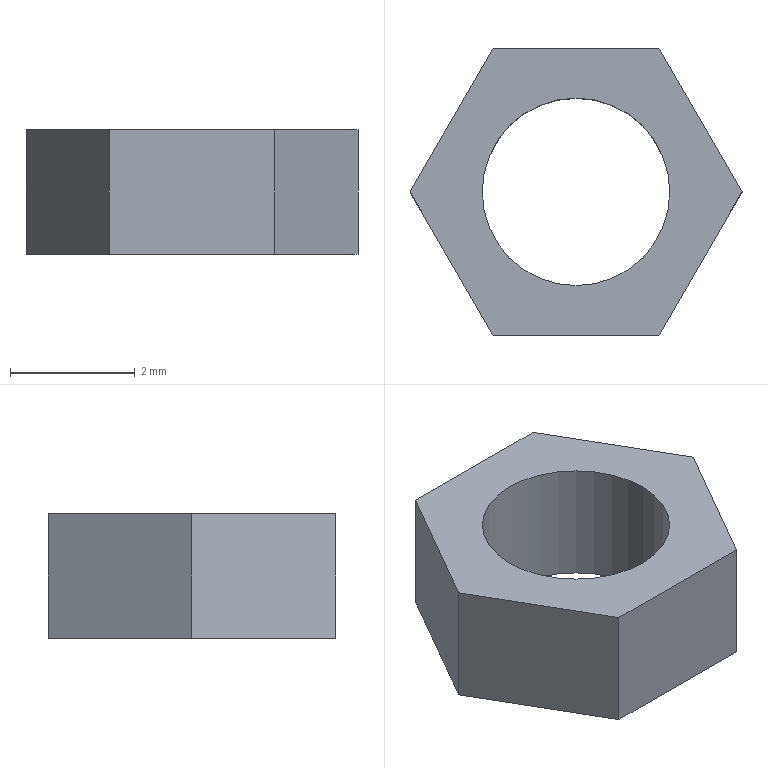Part | SolidWorks | features BaseBody 1 | 1 solid | 10 faces | box 5.314 x 4.602 x 2 mm | volume 22.552 mm3 | plane 8 | cylinder 2 | commonest cylinder face diameters 3 x2
STEP:
#1=CARTESIAN_POINT('',(35.309,0.,0.));
#2=VERTEX_POINT('',#1);
#3=CARTESIAN_POINT('',(38.309,0.,0.));
#4=VERTEX_POINT('',#3);
#5=CARTESIAN_POINT('',(36.809,0.,0.));
#6=DIRECTION('',(0.,0.,1.));
#7=DIRECTION('',(1.,0.,0.));
#8=AXIS2_PLACEMENT_3D('',#5,#6,#7);
#9=CIRCLE('',#8,1.5);
#10=EDGE_CURVE('',#2,#4,#9,.T.);
#11=ORIENTED_EDGE('',*,*,#10,.F.);
#12=CARTESIAN_POINT('',(35.309,0.,2.));
#13=VERTEX_POINT('',#12);
#14=CARTESIAN_POINT('',(35.309,0.,0.));
#15=DIRECTION('',(0.,0.,1.));
#16=VECTOR('',#15,1000.);
#17=LINE('',#14,#16);
#18=EDGE_CURVE('',#2,#13,#17,.T.);
#19=ORIENTED_EDGE('',*,*,#18,.T.);
#20=CARTESIAN_POINT('',(38.309,0.,2.));
#21=VERTEX_POINT('',#20);
#22=CARTESIAN_POINT('',(36.809,0.,2.));
#23=DIRECTION('',(0.,0.,-1.));
#24=DIRECTION('',(1.,0.,0.));
#25=AXIS2_PLACEMENT_3D('',#22,#23,#24);
#26=CIRCLE('',#25,1.5);
#27=EDGE_CURVE('',#21,#13,#26,.T.);
#28=ORIENTED_EDGE('',*,*,#27,.F.);
#29=CARTESIAN_POINT('',(38.309,0.,0.));
#30=DIRECTION('',(0.,0.,1.));
#31=VECTOR('',#30,1000.);
#32=LINE('',#29,#31);
#33=EDGE_CURVE('',#4,#21,#32,.T.);
#34=ORIENTED_EDGE('',*,*,#33,.F.);
#35=EDGE_LOOP('',(#11,#19,#28,#34));
#36=FACE_OUTER_BOUND('',#35,.T.);
#37=CARTESIAN_POINT('',(36.809,0.,0.));
#38=DIRECTION('',(0.,0.,1.));
#39=DIRECTION('',(1.,0.,0.));
#40=AXIS2_PLACEMENT_3D('',#37,#38,#39);
#41=CYLINDRICAL_SURFACE('',#40,1.5);
#42=ADVANCED_FACE('',(#36),#41,.F.);
#43=ORIENTED_EDGE('',*,*,#18,.F.);
#44=CARTESIAN_POINT('',(36.809,0.,0.));
#45=DIRECTION('',(0.,0.,1.));
#46=DIRECTION('',(1.,0.,0.));
#47=AXIS2_PLACEMENT_3D('',#44,#45,#46);
#48=CIRCLE('',#47,1.5);
#49=EDGE_CURVE('',#4,#2,#48,.T.);
#50=ORIENTED_EDGE('',*,*,#49,.F.);
#51=ORIENTED_EDGE('',*,*,#33,.T.);
#52=CARTESIAN_POINT('',(36.809,0.,2.));
#53=DIRECTION('',(0.,0.,-1.));
#54=DIRECTION('',(1.,0.,0.));
#55=AXIS2_PLACEMENT_3D('',#52,#53,#54);
#56=CIRCLE('',#55,1.5);
#57=EDGE_CURVE('',#13,#21,#56,.T.);
#58=ORIENTED_EDGE('',*,*,#57,.F.);
#59=EDGE_LOOP('',(#43,#50,#51,#58));
#60=FACE_OUTER_BOUND('',#59,.T.);
#61=CARTESIAN_POINT('',(36.809,0.,0.));
#62=DIRECTION('',(0.,0.,1.));
#63=DIRECTION('',(1.,0.,0.));
#64=AXIS2_PLACEMENT_3D('',#61,#62,#63);
#65=CYLINDRICAL_SURFACE('',#64,1.5);
#66=ADVANCED_FACE('',(#60),#65,.F.);
#67=ORIENTED_EDGE('',*,*,#27,.T.);
#68=ORIENTED_EDGE('',*,*,#57,.T.);
#69=EDGE_LOOP('',(#67,#68));
#70=FACE_BOUND('',#69,.T.);
#71=CARTESIAN_POINT('',(39.466,0.,2.));
#72=VERTEX_POINT('',#71);
#73=CARTESIAN_POINT('',(38.138,2.301,2.));
#74=VERTEX_POINT('',#73);
#75=CARTESIAN_POINT('',(39.466,0.,2.));
#76=DIRECTION('',(-0.5,0.866,0.));
#77=VECTOR('',#76,1000.);
#78=LINE('',#75,#77);
#79=EDGE_CURVE('',#72,#74,#78,.T.);
#80=ORIENTED_EDGE('',*,*,#79,.T.);
#81=CARTESIAN_POINT('',(35.48,2.301,2.));
#82=VERTEX_POINT('',#81);
#83=CARTESIAN_POINT('',(36.809,2.301,2.));
#84=DIRECTION('',(-1.,0.,0.));
#85=VECTOR('',#84,1000.);
#86=LINE('',#83,#85);
#87=EDGE_CURVE('',#74,#82,#86,.T.);
#88=ORIENTED_EDGE('',*,*,#87,.T.);
#89=CARTESIAN_POINT('',(34.152,0.,2.));
#90=VERTEX_POINT('',#89);
#91=CARTESIAN_POINT('',(35.48,2.301,2.));
#92=DIRECTION('',(-0.5,-0.866,0.));
#93=VECTOR('',#92,1000.);
#94=LINE('',#91,#93);
#95=EDGE_CURVE('',#82,#90,#94,.T.);
#96=ORIENTED_EDGE('',*,*,#95,.T.);
#97=CARTESIAN_POINT('',(35.48,-2.301,2.));
#98=VERTEX_POINT('',#97);
#99=CARTESIAN_POINT('',(34.152,0.,2.));
#100=DIRECTION('',(0.5,-0.866,0.));
#101=VECTOR('',#100,1000.);
#102=LINE('',#99,#101);
#103=EDGE_CURVE('',#90,#98,#102,.T.);
#104=ORIENTED_EDGE('',*,*,#103,.T.);
#105=CARTESIAN_POINT('',(38.138,-2.301,2.));
#106=VERTEX_POINT('',#105);
#107=CARTESIAN_POINT('',(36.809,-2.301,2.));
#108=DIRECTION('',(1.,0.,0.));
#109=VECTOR('',#108,1000.);
#110=LINE('',#107,#109);
#111=EDGE_CURVE('',#98,#106,#110,.T.);
#112=ORIENTED_EDGE('',*,*,#111,.T.);
#113=CARTESIAN_POINT('',(38.138,-2.301,2.));
#114=DIRECTION('',(0.5,0.866,0.));
#115=VECTOR('',#114,1000.);
#116=LINE('',#113,#115);
#117=EDGE_CURVE('',#106,#72,#116,.T.);
#118=ORIENTED_EDGE('',*,*,#117,.T.);
#119=EDGE_LOOP('',(#80,#88,#96,#104,#112,#118));
#120=FACE_OUTER_BOUND('',#119,.T.);
#121=CARTESIAN_POINT('',(36.809,0.,2.));
#122=DIRECTION('',(0.,0.,1.));
#123=DIRECTION('',(1.,0.,0.));
#124=AXIS2_PLACEMENT_3D('',#121,#122,#123);
#125=PLANE('',#124);
#126=ADVANCED_FACE('',(#70,#120),#125,.T.);
#127=ORIENTED_EDGE('',*,*,#49,.T.);
#128=ORIENTED_EDGE('',*,*,#10,.T.);
#129=EDGE_LOOP('',(#127,#128));
#130=FACE_BOUND('',#129,.T.);
#131=CARTESIAN_POINT('',(38.138,2.301,0.));
#132=VERTEX_POINT('',#131);
#133=CARTESIAN_POINT('',(35.48,2.301,0.));
#134=VERTEX_POINT('',#133);
#135=CARTESIAN_POINT('',(36.809,2.301,0.));
#136=DIRECTION('',(-1.,0.,0.));
#137=VECTOR('',#136,1000.);
#138=LINE('',#135,#137);
#139=EDGE_CURVE('',#132,#134,#138,.T.);
#140=ORIENTED_EDGE('',*,*,#139,.F.);
#141=CARTESIAN_POINT('',(39.466,0.,0.));
#142=VERTEX_POINT('',#141);
#143=CARTESIAN_POINT('',(39.466,0.,0.));
#144=DIRECTION('',(-0.5,0.866,0.));
#145=VECTOR('',#144,1000.);
#146=LINE('',#143,#145);
#147=EDGE_CURVE('',#142,#132,#146,.T.);
#148=ORIENTED_EDGE('',*,*,#147,.F.);
#149=CARTESIAN_POINT('',(38.138,-2.301,0.));
#150=VERTEX_POINT('',#149);
#151=CARTESIAN_POINT('',(38.138,-2.301,0.));
#152=DIRECTION('',(0.5,0.866,0.));
#153=VECTOR('',#152,1000.);
#154=LINE('',#151,#153);
#155=EDGE_CURVE('',#150,#142,#154,.T.);
#156=ORIENTED_EDGE('',*,*,#155,.F.);
#157=CARTESIAN_POINT('',(35.48,-2.301,0.));
#158=VERTEX_POINT('',#157);
#159=CARTESIAN_POINT('',(36.809,-2.301,0.));
#160=DIRECTION('',(1.,0.,0.));
#161=VECTOR('',#160,1000.);
#162=LINE('',#159,#161);
#163=EDGE_CURVE('',#158,#150,#162,.T.);
#164=ORIENTED_EDGE('',*,*,#163,.F.);
#165=CARTESIAN_POINT('',(34.152,0.,0.));
#166=VERTEX_POINT('',#165);
#167=CARTESIAN_POINT('',(34.152,0.,0.));
#168=DIRECTION('',(0.5,-0.866,0.));
#169=VECTOR('',#168,1000.);
#170=LINE('',#167,#169);
#171=EDGE_CURVE('',#166,#158,#170,.T.);
#172=ORIENTED_EDGE('',*,*,#171,.F.);
#173=CARTESIAN_POINT('',(35.48,2.301,0.));
#174=DIRECTION('',(-0.5,-0.866,0.));
#175=VECTOR('',#174,1000.);
#176=LINE('',#173,#175);
#177=EDGE_CURVE('',#134,#166,#176,.T.);
#178=ORIENTED_EDGE('',*,*,#177,.F.);
#179=EDGE_LOOP('',(#140,#148,#156,#164,#172,#178));
#180=FACE_OUTER_BOUND('',#179,.T.);
#181=CARTESIAN_POINT('',(36.809,0.,0.));
#182=DIRECTION('',(0.,0.,1.));
#183=DIRECTION('',(1.,0.,0.));
#184=AXIS2_PLACEMENT_3D('',#181,#182,#183);
#185=PLANE('',#184);
#186=ADVANCED_FACE('',(#130,#180),#185,.F.);
#187=ORIENTED_EDGE('',*,*,#87,.F.);
#188=CARTESIAN_POINT('',(38.138,2.301,0.));
#189=DIRECTION('',(0.,0.,-1.));
#190=VECTOR('',#189,1000.);
#191=LINE('',#188,#190);
#192=EDGE_CURVE('',#74,#132,#191,.T.);
#193=ORIENTED_EDGE('',*,*,#192,.T.);
#194=ORIENTED_EDGE('',*,*,#139,.T.);
#195=CARTESIAN_POINT('',(35.48,2.301,0.));
#196=DIRECTION('',(0.,0.,1.));
#197=VECTOR('',#196,1000.);
#198=LINE('',#195,#197);
#199=EDGE_CURVE('',#134,#82,#198,.T.);
#200=ORIENTED_EDGE('',*,*,#199,.T.);
#201=EDGE_LOOP('',(#187,#193,#194,#200));
#202=FACE_OUTER_BOUND('',#201,.T.);
#203=CARTESIAN_POINT('',(38.138,2.301,0.));
#204=DIRECTION('',(0.,1.,0.));
#205=DIRECTION('',(0.,0.,1.));
#206=AXIS2_PLACEMENT_3D('',#203,#204,#205);
#207=PLANE('',#206);
#208=ADVANCED_FACE('',(#202),#207,.T.);
#209=ORIENTED_EDGE('',*,*,#79,.F.);
#210=CARTESIAN_POINT('',(39.466,0.,0.));
#211=DIRECTION('',(0.,0.,-1.));
#212=VECTOR('',#211,1000.);
#213=LINE('',#210,#212);
#214=EDGE_CURVE('',#72,#142,#213,.T.);
#215=ORIENTED_EDGE('',*,*,#214,.T.);
#216=ORIENTED_EDGE('',*,*,#147,.T.);
#217=ORIENTED_EDGE('',*,*,#192,.F.);
#218=EDGE_LOOP('',(#209,#215,#216,#217));
#219=FACE_OUTER_BOUND('',#218,.T.);
#220=CARTESIAN_POINT('',(39.466,0.,0.));
#221=DIRECTION('',(0.866,0.5,0.));
#222=DIRECTION('',(-0.5,0.866,0.));
#223=AXIS2_PLACEMENT_3D('',#220,#221,#222);
#224=PLANE('',#223);
#225=ADVANCED_FACE('',(#219),#224,.T.);
#226=ORIENTED_EDGE('',*,*,#117,.F.);
#227=CARTESIAN_POINT('',(38.138,-2.301,0.));
#228=DIRECTION('',(0.,0.,-1.));
#229=VECTOR('',#228,1000.);
#230=LINE('',#227,#229);
#231=EDGE_CURVE('',#106,#150,#230,.T.);
#232=ORIENTED_EDGE('',*,*,#231,.T.);
#233=ORIENTED_EDGE('',*,*,#155,.T.);
#234=ORIENTED_EDGE('',*,*,#214,.F.);
#235=EDGE_LOOP('',(#226,#232,#233,#234));
#236=FACE_OUTER_BOUND('',#235,.T.);
#237=CARTESIAN_POINT('',(38.138,-2.301,0.));
#238=DIRECTION('',(0.866,-0.5,0.));
#239=DIRECTION('',(0.5,0.866,0.));
#240=AXIS2_PLACEMENT_3D('',#237,#238,#239);
#241=PLANE('',#240);
#242=ADVANCED_FACE('',(#236),#241,.T.);
#243=ORIENTED_EDGE('',*,*,#111,.F.);
#244=CARTESIAN_POINT('',(35.48,-2.301,0.));
#245=DIRECTION('',(0.,0.,-1.));
#246=VECTOR('',#245,1000.);
#247=LINE('',#244,#246);
#248=EDGE_CURVE('',#98,#158,#247,.T.);
#249=ORIENTED_EDGE('',*,*,#248,.T.);
#250=ORIENTED_EDGE('',*,*,#163,.T.);
#251=ORIENTED_EDGE('',*,*,#231,.F.);
#252=EDGE_LOOP('',(#243,#249,#250,#251));
#253=FACE_OUTER_BOUND('',#252,.T.);
#254=CARTESIAN_POINT('',(35.48,-2.301,0.));
#255=DIRECTION('',(0.,-1.,0.));
#256=DIRECTION('',(0.,0.,-1.));
#257=AXIS2_PLACEMENT_3D('',#254,#255,#256);
#258=PLANE('',#257);
#259=ADVANCED_FACE('',(#253),#258,.T.);
#260=ORIENTED_EDGE('',*,*,#103,.F.);
#261=CARTESIAN_POINT('',(34.152,0.,0.));
#262=DIRECTION('',(0.,0.,-1.));
#263=VECTOR('',#262,1000.);
#264=LINE('',#261,#263);
#265=EDGE_CURVE('',#90,#166,#264,.T.);
#266=ORIENTED_EDGE('',*,*,#265,.T.);
#267=ORIENTED_EDGE('',*,*,#171,.T.);
#268=ORIENTED_EDGE('',*,*,#248,.F.);
#269=EDGE_LOOP('',(#260,#266,#267,#268));
#270=FACE_OUTER_BOUND('',#269,.T.);
#271=CARTESIAN_POINT('',(34.152,0.,0.));
#272=DIRECTION('',(-0.866,-0.5,0.));
#273=DIRECTION('',(0.5,-0.866,0.));
#274=AXIS2_PLACEMENT_3D('',#271,#272,#273);
#275=PLANE('',#274);
#276=ADVANCED_FACE('',(#270),#275,.T.);
#277=ORIENTED_EDGE('',*,*,#95,.F.);
#278=ORIENTED_EDGE('',*,*,#199,.F.);
#279=ORIENTED_EDGE('',*,*,#177,.T.);
#280=ORIENTED_EDGE('',*,*,#265,.F.);
#281=EDGE_LOOP('',(#277,#278,#279,#280));
#282=FACE_OUTER_BOUND('',#281,.T.);
#283=CARTESIAN_POINT('',(35.48,2.301,0.));
#284=DIRECTION('',(-0.866,0.5,0.));
#285=DIRECTION('',(-0.5,-0.866,0.));
#286=AXIS2_PLACEMENT_3D('',#283,#284,#285);
#287=PLANE('',#286);
#288=ADVANCED_FACE('',(#282),#287,.T.);
#289=CLOSED_SHELL('',(#42,#66,#126,#186,#208,#225,#242,#259,#276,#288));
#290=MANIFOLD_SOLID_BREP('',#289);
#291=CARTESIAN_POINT('',(0.,0.,0.));
#292=DIRECTION('',(0.,0.,1.));
#293=DIRECTION('',(1.,0.,0.));
#294=AXIS2_PLACEMENT_3D('',#291,#292,#293);
#295=(LENGTH_UNIT()NAMED_UNIT(*)SI_UNIT(.MILLI.,.METRE.));
#296=UNCERTAINTY_MEASURE_WITH_UNIT(LENGTH_MEASURE(0.00001),#295,'','');
#297=(NAMED_UNIT(*)PLANE_ANGLE_UNIT()SI_UNIT($,.RADIAN.));
#298=(NAMED_UNIT(*)SI_UNIT($,.STERADIAN.)SOLID_ANGLE_UNIT());
#299=(GEOMETRIC_REPRESENTATION_CONTEXT(3)GLOBAL_UNCERTAINTY_ASSIGNED_CONTEXT((#296))GLOBAL_UNIT_ASSIGNED_CONTEXT((#295,#297,#298))REPRESENTATION_CONTEXT('',''));
#300=ADVANCED_BREP_SHAPE_REPRESENTATION('',(#290,#294),#299);